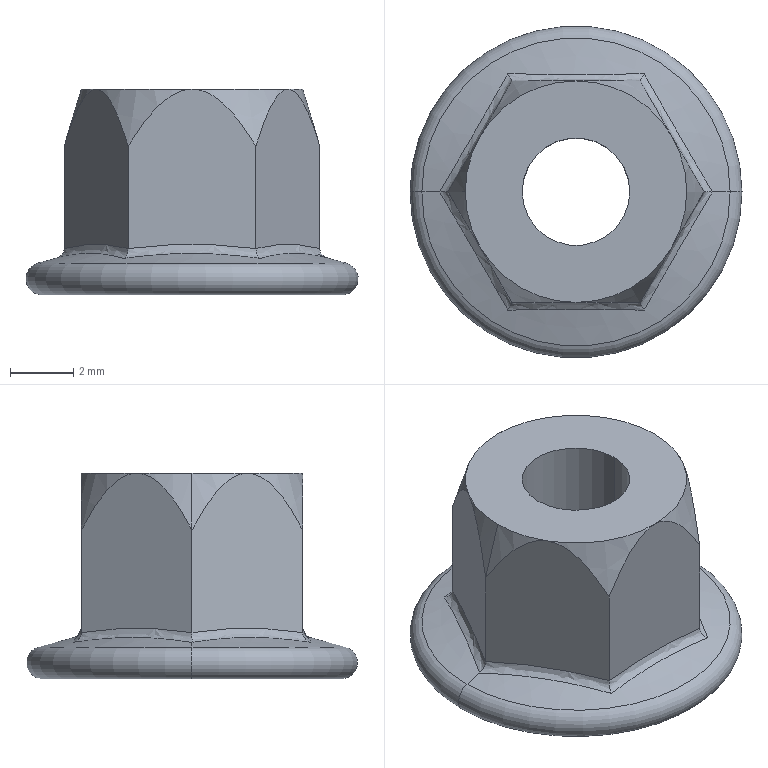Part | SolidWorks | features RevCut 2, Chamfer 1, Cut 1, Extrusion 1, Fillet 1, LPattern 1, Revolution 1 | 1 solid | 29 faces | box 10.5 x 10.5 x 6.5 mm | volume 259.355 mm3 | cone 11 | plane 8 | spline 6 | torus 2 | cylinder 2 | commonest cylinder face diameters 3.4 x2
STEP:
#1=CARTESIAN_POINT('',(2.155,3.733,-5.349));
#2=VERTEX_POINT('',#1);
#3=CARTESIAN_POINT('',(4.31,0.,-5.349));
#4=VERTEX_POINT('',#3);
#5=CARTESIAN_POINT('',(2.155,3.733,-5.349));
#6=CARTESIAN_POINT('',(2.508,3.111,-5.252));
#7=CARTESIAN_POINT('',(2.862,2.487,-5.192));
#8=CARTESIAN_POINT('',(3.584,1.237,-5.192));
#9=CARTESIAN_POINT('',(3.948,0.6165,-5.252));
#10=CARTESIAN_POINT('',(4.31,0.,-5.349));
#11=B_SPLINE_CURVE_WITH_KNOTS('',3,(#5,#6,#7,#8,#9,#10),.UNSPECIFIED.,.F.,.F.,(4,2,4),(0.,0.00216,0.004319),.UNSPECIFIED.);
#12=EDGE_CURVE('',#2,#4,#11,.T.);
#13=ORIENTED_EDGE('',*,*,#12,.T.);
#14=CARTESIAN_POINT('',(4.873,0.,-5.5));
#15=VERTEX_POINT('',#14);
#16=CARTESIAN_POINT('',(4.041,0.,-5.277));
#17=DIRECTION('',(0.9659,0.,-0.2588));
#18=VECTOR('',#17,1000.);
#19=LINE('',#16,#18);
#20=EDGE_CURVE('',#4,#15,#19,.T.);
#21=ORIENTED_EDGE('',*,*,#20,.T.);
#22=CARTESIAN_POINT('',(-4.873,0.,-5.5));
#23=VERTEX_POINT('',#22);
#24=CARTESIAN_POINT('',(0.,0.,-5.5));
#25=DIRECTION('',(0.,0.,-1.));
#26=DIRECTION('',(-1.,0.,0.));
#27=AXIS2_PLACEMENT_3D('',#24,#25,#26);
#28=CIRCLE('',#27,4.873);
#29=EDGE_CURVE('',#23,#15,#28,.T.);
#30=ORIENTED_EDGE('',*,*,#29,.F.);
#31=CARTESIAN_POINT('',(-4.31,0.,-5.349));
#32=VERTEX_POINT('',#31);
#33=CARTESIAN_POINT('',(-4.041,0.,-5.277));
#34=DIRECTION('',(-0.9659,0.,-0.2588));
#35=VECTOR('',#34,1000.);
#36=LINE('',#33,#35);
#37=EDGE_CURVE('',#32,#23,#36,.T.);
#38=ORIENTED_EDGE('',*,*,#37,.F.);
#39=CARTESIAN_POINT('',(-2.155,3.733,-5.349));
#40=VERTEX_POINT('',#39);
#41=CARTESIAN_POINT('',(-4.31,0.,-5.349));
#42=CARTESIAN_POINT('',(-3.948,0.6162,-5.252));
#43=CARTESIAN_POINT('',(-3.585,1.235,-5.192));
#44=CARTESIAN_POINT('',(-2.863,2.485,-5.192));
#45=CARTESIAN_POINT('',(-2.508,3.111,-5.252));
#46=CARTESIAN_POINT('',(-2.155,3.733,-5.349));
#47=B_SPLINE_CURVE_WITH_KNOTS('',3,(#41,#42,#43,#44,#45,#46),.UNSPECIFIED.,.F.,.F.,(4,2,4),(0.,0.00216,0.004319),.UNSPECIFIED.);
#48=EDGE_CURVE('',#32,#40,#47,.T.);
#49=ORIENTED_EDGE('',*,*,#48,.T.);
#50=CARTESIAN_POINT('',(-2.155,3.733,-5.349));
#51=CARTESIAN_POINT('',(-1.44,3.727,-5.252));
#52=CARTESIAN_POINT('',(-0.7231,3.722,-5.192));
#53=CARTESIAN_POINT('',(0.7205,3.722,-5.192));
#54=CARTESIAN_POINT('',(1.44,3.727,-5.252));
#55=CARTESIAN_POINT('',(2.155,3.733,-5.349));
#56=B_SPLINE_CURVE_WITH_KNOTS('',3,(#50,#51,#52,#53,#54,#55),.UNSPECIFIED.,.F.,.F.,(4,2,4),(0.,0.00216,0.004319),.UNSPECIFIED.);
#57=EDGE_CURVE('',#40,#2,#56,.T.);
#58=ORIENTED_EDGE('',*,*,#57,.T.);
#59=EDGE_LOOP('',(#13,#21,#30,#38,#49,#58));
#60=FACE_OUTER_BOUND('',#59,.T.);
#61=CARTESIAN_POINT('',(0.,0.,-5.277));
#62=DIRECTION('',(0.,0.,-1.));
#63=DIRECTION('',(-1.,0.,0.));
#64=AXIS2_PLACEMENT_3D('',#61,#62,#63);
#65=CONICAL_SURFACE('',#64,4.041,1.309);
#66=ADVANCED_FACE('',(#60),#65,.T.);
#67=ORIENTED_EDGE('',*,*,#29,.T.);
#68=CARTESIAN_POINT('',(4.741,0.,-6.5));
#69=VERTEX_POINT('',#68);
#70=CARTESIAN_POINT('',(4.741,0.,-5.991));
#71=DIRECTION('',(0.,1.,0.));
#72=DIRECTION('',(-1.,0.,0.));
#73=AXIS2_PLACEMENT_3D('',#70,#71,#72);
#74=CIRCLE('',#73,0.5087);
#75=EDGE_CURVE('',#15,#69,#74,.T.);
#76=ORIENTED_EDGE('',*,*,#75,.T.);
#77=CARTESIAN_POINT('',(-4.741,0.,-6.5));
#78=VERTEX_POINT('',#77);
#79=CARTESIAN_POINT('',(0.,0.,-6.5));
#80=DIRECTION('',(0.,0.,-1.));
#81=DIRECTION('',(-1.,0.,0.));
#82=AXIS2_PLACEMENT_3D('',#79,#80,#81);
#83=CIRCLE('',#82,4.741);
#84=EDGE_CURVE('',#78,#69,#83,.T.);
#85=ORIENTED_EDGE('',*,*,#84,.F.);
#86=CARTESIAN_POINT('',(-4.741,0.,-5.991));
#87=DIRECTION('',(0.,-1.,0.));
#88=DIRECTION('',(0.,0.,-1.));
#89=AXIS2_PLACEMENT_3D('',#86,#87,#88);
#90=CIRCLE('',#89,0.5087);
#91=EDGE_CURVE('',#23,#78,#90,.T.);
#92=ORIENTED_EDGE('',*,*,#91,.F.);
#93=EDGE_LOOP('',(#67,#76,#85,#92));
#94=FACE_OUTER_BOUND('',#93,.T.);
#95=CARTESIAN_POINT('',(0.,0.,-5.991));
#96=DIRECTION('',(0.,0.,-1.));
#97=DIRECTION('',(-1.,0.,0.));
#98=AXIS2_PLACEMENT_3D('',#95,#96,#97);
#99=TOROIDAL_SURFACE('',#98,4.741,0.5087);
#100=ADVANCED_FACE('',(#94),#99,.T.);
#101=CARTESIAN_POINT('',(1.7,0.,-6.014));
#102=VERTEX_POINT('',#101);
#103=CARTESIAN_POINT('',(-1.7,0.,-6.014));
#104=VERTEX_POINT('',#103);
#105=CARTESIAN_POINT('',(0.,0.,-6.014));
#106=DIRECTION('',(0.,0.,-1.));
#107=DIRECTION('',(1.,0.,0.));
#108=AXIS2_PLACEMENT_3D('',#105,#106,#107);
#109=CIRCLE('',#108,1.7);
#110=EDGE_CURVE('',#102,#104,#109,.T.);
#111=ORIENTED_EDGE('',*,*,#110,.F.);
#112=CARTESIAN_POINT('',(2.186,0.,-6.5));
#113=VERTEX_POINT('',#112);
#114=CARTESIAN_POINT('',(2.186,0.,-6.5));
#115=DIRECTION('',(0.7071,0.,-0.7071));
#116=VECTOR('',#115,1000.);
#117=LINE('',#114,#116);
#118=EDGE_CURVE('',#102,#113,#117,.T.);
#119=ORIENTED_EDGE('',*,*,#118,.T.);
#120=CARTESIAN_POINT('',(-2.186,0.,-6.5));
#121=VERTEX_POINT('',#120);
#122=CARTESIAN_POINT('',(0.,0.,-6.5));
#123=DIRECTION('',(0.,0.,1.));
#124=DIRECTION('',(1.,0.,0.));
#125=AXIS2_PLACEMENT_3D('',#122,#123,#124);
#126=CIRCLE('',#125,2.186);
#127=EDGE_CURVE('',#121,#113,#126,.T.);
#128=ORIENTED_EDGE('',*,*,#127,.F.);
#129=CARTESIAN_POINT('',(-2.186,0.,-6.5));
#130=DIRECTION('',(-0.7071,0.,-0.7071));
#131=VECTOR('',#130,1000.);
#132=LINE('',#129,#131);
#133=EDGE_CURVE('',#104,#121,#132,.T.);
#134=ORIENTED_EDGE('',*,*,#133,.F.);
#135=EDGE_LOOP('',(#111,#119,#128,#134));
#136=FACE_OUTER_BOUND('',#135,.T.);
#137=CARTESIAN_POINT('',(0.,0.,-6.5));
#138=DIRECTION('',(0.,0.,-1.));
#139=DIRECTION('',(-1.,0.,0.));
#140=AXIS2_PLACEMENT_3D('',#137,#138,#139);
#141=CONICAL_SURFACE('',#140,2.186,0.7854);
#142=ADVANCED_FACE('',(#136),#141,.F.);
#143=ORIENTED_EDGE('',*,*,#110,.T.);
#144=CARTESIAN_POINT('',(-1.7,0.,0.));
#145=VERTEX_POINT('',#144);
#146=CARTESIAN_POINT('',(-1.7,0.,-6.5));
#147=DIRECTION('',(0.,0.,1.));
#148=VECTOR('',#147,1000.);
#149=LINE('',#146,#148);
#150=EDGE_CURVE('',#104,#145,#149,.T.);
#151=ORIENTED_EDGE('',*,*,#150,.T.);
#152=CARTESIAN_POINT('',(1.7,0.,0.));
#153=VERTEX_POINT('',#152);
#154=CARTESIAN_POINT('',(0.,0.,0.));
#155=DIRECTION('',(0.,0.,1.));
#156=DIRECTION('',(1.,0.,0.));
#157=AXIS2_PLACEMENT_3D('',#154,#155,#156);
#158=CIRCLE('',#157,1.7);
#159=EDGE_CURVE('',#145,#153,#158,.T.);
#160=ORIENTED_EDGE('',*,*,#159,.T.);
#161=CARTESIAN_POINT('',(1.7,0.,-6.5));
#162=DIRECTION('',(0.,0.,1.));
#163=VECTOR('',#162,1000.);
#164=LINE('',#161,#163);
#165=EDGE_CURVE('',#102,#153,#164,.T.);
#166=ORIENTED_EDGE('',*,*,#165,.F.);
#167=EDGE_LOOP('',(#143,#151,#160,#166));
#168=FACE_OUTER_BOUND('',#167,.T.);
#169=CARTESIAN_POINT('',(0.,0.,-6.5));
#170=DIRECTION('',(0.,0.,1.));
#171=DIRECTION('',(1.,0.,0.));
#172=AXIS2_PLACEMENT_3D('',#169,#170,#171);
#173=CYLINDRICAL_SURFACE('',#172,1.7);
#174=ADVANCED_FACE('',(#168),#173,.F.);
#175=CARTESIAN_POINT('',(-3.031,-1.75,0.));
#176=VERTEX_POINT('',#175);
#177=CARTESIAN_POINT('',(-3.5,0.,0.));
#178=VERTEX_POINT('',#177);
#179=CARTESIAN_POINT('',(0.,0.,0.));
#180=DIRECTION('',(0.,0.,-1.));
#181=DIRECTION('',(1.,0.,0.));
#182=AXIS2_PLACEMENT_3D('',#179,#180,#181);
#183=CIRCLE('',#182,3.5);
#184=EDGE_CURVE('',#176,#178,#183,.T.);
#185=ORIENTED_EDGE('',*,*,#184,.T.);
#186=CARTESIAN_POINT('',(-4.041,0.,-1.8));
#187=VERTEX_POINT('',#186);
#188=CARTESIAN_POINT('',(-3.5,0.,0.));
#189=DIRECTION('',(-0.2881,0.,-0.9576));
#190=VECTOR('',#189,1000.);
#191=LINE('',#188,#190);
#192=EDGE_CURVE('',#178,#187,#191,.T.);
#193=ORIENTED_EDGE('',*,*,#192,.T.);
#194=CARTESIAN_POINT('',(-4.041,0.,-1.8));
#195=CARTESIAN_POINT('',(-3.981,-0.1048,-1.599));
#196=CARTESIAN_POINT('',(-3.918,-0.2143,-1.402));
#197=CARTESIAN_POINT('',(-3.783,-0.4485,-1.021));
#198=CARTESIAN_POINT('',(-3.711,-0.5729,-0.8364));
#199=CARTESIAN_POINT('',(-3.551,-0.8499,-0.4918));
#200=CARTESIAN_POINT('',(-3.463,-1.002,-0.3309));
#201=CARTESIAN_POINT('',(-3.313,-1.262,-0.1453));
#202=CARTESIAN_POINT('',(-3.26,-1.353,-0.09372));
#203=CARTESIAN_POINT('',(-3.149,-1.546,-0.02051));
#204=CARTESIAN_POINT('',(-3.09,-1.648,0.));
#205=CARTESIAN_POINT('',(-3.031,-1.75,0.));
#206=B_SPLINE_CURVE_WITH_KNOTS('',3,(#194,#195,#196,#197,#198,#199,#200,#201,#202,#203,#204,#205),.UNSPECIFIED.,.F.,.F.,(4,2,2,2,2,4),(0.000000232,0.0007011,0.001402,0.002103,0.002453,0.002804),.UNSPECIFIED.);
#207=EDGE_CURVE('',#187,#176,#206,.T.);
#208=ORIENTED_EDGE('',*,*,#207,.T.);
#209=EDGE_LOOP('',(#185,#193,#208));
#210=FACE_OUTER_BOUND('',#209,.T.);
#211=CARTESIAN_POINT('',(0.,0.,0.));
#212=DIRECTION('',(0.,0.,-1.));
#213=DIRECTION('',(-1.,0.,0.));
#214=AXIS2_PLACEMENT_3D('',#211,#212,#213);
#215=CONICAL_SURFACE('',#214,3.5,0.2922);
#216=ADVANCED_FACE('',(#210),#215,.T.);
#217=CARTESIAN_POINT('',(2.021,-3.5,-5.037));
#218=VERTEX_POINT('',#217);
#219=CARTESIAN_POINT('',(2.021,-3.5,-1.8));
#220=VERTEX_POINT('',#219);
#221=CARTESIAN_POINT('',(2.021,-3.5,-6.5));
#222=DIRECTION('',(0.,0.,1.));
#223=VECTOR('',#222,1000.);
#224=LINE('',#221,#223);
#225=EDGE_CURVE('',#218,#220,#224,.T.);
#226=ORIENTED_EDGE('',*,*,#225,.F.);
#227=CARTESIAN_POINT('',(4.041,0.,-5.037));
#228=VERTEX_POINT('',#227);
#229=CARTESIAN_POINT('',(2.021,-3.5,-5.037));
#230=CARTESIAN_POINT('',(2.356,-2.919,-4.953));
#231=CARTESIAN_POINT('',(2.693,-2.336,-4.902));
#232=CARTESIAN_POINT('',(3.369,-1.164,-4.902));
#233=CARTESIAN_POINT('',(3.706,-0.5811,-4.953));
#234=CARTESIAN_POINT('',(4.041,0.,-5.037));
#235=B_SPLINE_CURVE_WITH_KNOTS('',3,(#229,#230,#231,#232,#233,#234),.UNSPECIFIED.,.F.,.F.,(4,2,4),(0.,0.002025,0.00405),.UNSPECIFIED.);
#236=EDGE_CURVE('',#218,#228,#235,.T.);
#237=ORIENTED_EDGE('',*,*,#236,.T.);
#238=CARTESIAN_POINT('',(4.041,0.,-1.8));
#239=VERTEX_POINT('',#238);
#240=CARTESIAN_POINT('',(4.041,0.,-6.5));
#241=DIRECTION('',(0.,0.,1.));
#242=VECTOR('',#241,1000.);
#243=LINE('',#240,#242);
#244=EDGE_CURVE('',#228,#239,#243,.T.);
#245=ORIENTED_EDGE('',*,*,#244,.T.);
#246=CARTESIAN_POINT('',(3.031,-1.75,0.));
#247=VERTEX_POINT('',#246);
#248=CARTESIAN_POINT('',(3.031,-1.75,0.));
#249=CARTESIAN_POINT('',(3.09,-1.648,0.));
#250=CARTESIAN_POINT('',(3.149,-1.545,-0.02068));
#251=CARTESIAN_POINT('',(3.262,-1.351,-0.09464));
#252=CARTESIAN_POINT('',(3.315,-1.258,-0.148));
#253=CARTESIAN_POINT('',(3.465,-0.9986,-0.3345));
#254=CARTESIAN_POINT('',(3.553,-0.8457,-0.4965));
#255=CARTESIAN_POINT('',(3.712,-0.571,-0.8393));
#256=CARTESIAN_POINT('',(3.783,-0.4472,-1.023));
#257=CARTESIAN_POINT('',(3.918,-0.2138,-1.403));
#258=CARTESIAN_POINT('',(3.981,-0.1046,-1.599));
#259=CARTESIAN_POINT('',(4.041,0.,-1.8));
#260=B_SPLINE_CURVE_WITH_KNOTS('',3,(#248,#249,#250,#251,#252,#253,#254,#255,#256,#257,#258,#259),.UNSPECIFIED.,.F.,.F.,(4,2,2,2,2,4),(0.002804,0.003155,0.003507,0.00421,0.004914,0.005617),.UNSPECIFIED.);
#261=EDGE_CURVE('',#247,#239,#260,.T.);
#262=ORIENTED_EDGE('',*,*,#261,.F.);
#263=CARTESIAN_POINT('',(2.021,-3.5,-1.8));
#264=CARTESIAN_POINT('',(2.081,-3.395,-1.599));
#265=CARTESIAN_POINT('',(2.144,-3.286,-1.402));
#266=CARTESIAN_POINT('',(2.28,-3.052,-1.021));
#267=CARTESIAN_POINT('',(2.351,-2.927,-0.8364));
#268=CARTESIAN_POINT('',(2.511,-2.65,-0.4918));
#269=CARTESIAN_POINT('',(2.599,-2.498,-0.3309));
#270=CARTESIAN_POINT('',(2.749,-2.238,-0.1453));
#271=CARTESIAN_POINT('',(2.802,-2.147,-0.09372));
#272=CARTESIAN_POINT('',(2.913,-1.954,-0.02051));
#273=CARTESIAN_POINT('',(2.972,-1.852,0.));
#274=CARTESIAN_POINT('',(3.031,-1.75,0.));
#275=B_SPLINE_CURVE_WITH_KNOTS('',3,(#263,#264,#265,#266,#267,#268,#269,#270,#271,#272,#273,#274),.UNSPECIFIED.,.F.,.F.,(4,2,2,2,2,4),(0.000000232,0.0007011,0.001402,0.002103,0.002453,0.002804),.UNSPECIFIED.);
#276=EDGE_CURVE('',#220,#247,#275,.T.);
#277=ORIENTED_EDGE('',*,*,#276,.F.);
#278=EDGE_LOOP('',(#226,#237,#245,#262,#277));
#279=FACE_OUTER_BOUND('',#278,.T.);
#280=CARTESIAN_POINT('',(2.021,-3.5,-6.5));
#281=DIRECTION('',(0.866,-0.5,0.));
#282=DIRECTION('',(0.5,0.866,0.));
#283=AXIS2_PLACEMENT_3D('',#280,#281,#282);
#284=PLANE('',#283);
#285=ADVANCED_FACE('',(#279),#284,.T.);
#286=CARTESIAN_POINT('',(-2.021,-3.5,-5.037));
#287=VERTEX_POINT('',#286);
#288=CARTESIAN_POINT('',(-2.021,-3.5,-1.8));
#289=VERTEX_POINT('',#288);
#290=CARTESIAN_POINT('',(-2.021,-3.5,-6.5));
#291=DIRECTION('',(0.,0.,1.));
#292=VECTOR('',#291,1000.);
#293=LINE('',#290,#292);
#294=EDGE_CURVE('',#287,#289,#293,.T.);
#295=ORIENTED_EDGE('',*,*,#294,.F.);
#296=CARTESIAN_POINT('',(-2.021,-3.5,-5.037));
#297=CARTESIAN_POINT('',(-1.35,-3.5,-4.953));
#298=CARTESIAN_POINT('',(-0.6766,-3.5,-4.902));
#299=CARTESIAN_POINT('',(0.6766,-3.5,-4.902));
#300=CARTESIAN_POINT('',(1.35,-3.5,-4.953));
#301=CARTESIAN_POINT('',(2.021,-3.5,-5.037));
#302=B_SPLINE_CURVE_WITH_KNOTS('',3,(#296,#297,#298,#299,#300,#301),.UNSPECIFIED.,.F.,.F.,(4,2,4),(0.,0.002025,0.00405),.UNSPECIFIED.);
#303=EDGE_CURVE('',#287,#218,#302,.T.);
#304=ORIENTED_EDGE('',*,*,#303,.T.);
#305=ORIENTED_EDGE('',*,*,#225,.T.);
#306=CARTESIAN_POINT('',(0.,-3.5,0.));
#307=VERTEX_POINT('',#306);
#308=CARTESIAN_POINT('',(0.,-3.5,0.));
#309=CARTESIAN_POINT('',(0.118,-3.5,0.));
#310=CARTESIAN_POINT('',(0.234,-3.5,-0.01997));
#311=CARTESIAN_POINT('',(0.4599,-3.5,-0.09407));
#312=CARTESIAN_POINT('',(0.5651,-3.5,-0.1462));
#313=CARTESIAN_POINT('',(0.7651,-3.5,-0.2703));
#314=CARTESIAN_POINT('',(0.8598,-3.5,-0.3426));
#315=CARTESIAN_POINT('',(1.037,-3.5,-0.4965));
#316=CARTESIAN_POINT('',(1.12,-3.5,-0.5787));
#317=CARTESIAN_POINT('',(1.359,-3.5,-0.8363));
#318=CARTESIAN_POINT('',(1.505,-3.5,-1.023));
#319=CARTESIAN_POINT('',(1.775,-3.5,-1.405));
#320=CARTESIAN_POINT('',(1.901,-3.5,-1.601));
#321=CARTESIAN_POINT('',(2.021,-3.5,-1.8));
#322=B_SPLINE_CURVE_WITH_KNOTS('',3,(#308,#309,#310,#311,#312,#313,#314,#315,#316,#317,#318,#319,#320,#321),.UNSPECIFIED.,.F.,.F.,(4,2,2,2,2,2,4),(0.00757,0.007919,0.008268,0.008616,0.008965,0.009663,0.01036),.UNSPECIFIED.);
#323=EDGE_CURVE('',#307,#220,#322,.T.);
#324=ORIENTED_EDGE('',*,*,#323,.F.);
#325=CARTESIAN_POINT('',(-2.021,-3.5,-1.8));
#326=CARTESIAN_POINT('',(-1.901,-3.5,-1.6));
#327=CARTESIAN_POINT('',(-1.774,-3.5,-1.403));
#328=CARTESIAN_POINT('',(-1.502,-3.5,-1.02));
#329=CARTESIAN_POINT('',(-1.358,-3.5,-0.8356));
#330=CARTESIAN_POINT('',(-1.04,-3.5,-0.4928));
#331=CARTESIAN_POINT('',(-0.8644,-3.5,-0.3318));
#332=CARTESIAN_POINT('',(-0.5645,-3.5,-0.1458));
#333=CARTESIAN_POINT('',(-0.4572,-3.5,-0.0931));
#334=CARTESIAN_POINT('',(-0.2354,-3.5,-0.02053));
#335=CARTESIAN_POINT('',(-0.1178,-3.5,0.));
#336=CARTESIAN_POINT('',(0.,-3.5,0.));
#337=B_SPLINE_CURVE_WITH_KNOTS('',3,(#325,#326,#327,#328,#329,#330,#331,#332,#333,#334,#335,#336),.UNSPECIFIED.,.F.,.F.,(4,2,2,2,2,4),(0.004785,0.005481,0.006177,0.006874,0.007222,0.00757),.UNSPECIFIED.);
#338=EDGE_CURVE('',#289,#307,#337,.T.);
#339=ORIENTED_EDGE('',*,*,#338,.F.);
#340=EDGE_LOOP('',(#295,#304,#305,#324,#339));
#341=FACE_OUTER_BOUND('',#340,.T.);
#342=CARTESIAN_POINT('',(-2.021,-3.5,-6.5));
#343=DIRECTION('',(0.,-1.,0.));
#344=DIRECTION('',(1.,0.,0.));
#345=AXIS2_PLACEMENT_3D('',#342,#343,#344);
#346=PLANE('',#345);
#347=ADVANCED_FACE('',(#341),#346,.T.);
#348=CARTESIAN_POINT('',(-4.041,0.,-5.037));
#349=VERTEX_POINT('',#348);
#350=CARTESIAN_POINT('',(-4.041,0.,-6.5));
#351=DIRECTION('',(0.,0.,1.));
#352=VECTOR('',#351,1000.);
#353=LINE('',#350,#352);
#354=EDGE_CURVE('',#349,#187,#353,.T.);
#355=ORIENTED_EDGE('',*,*,#354,.F.);
#356=CARTESIAN_POINT('',(-4.041,0.,-5.037));
#357=CARTESIAN_POINT('',(-3.706,-0.5811,-4.953));
#358=CARTESIAN_POINT('',(-3.369,-1.164,-4.902));
#359=CARTESIAN_POINT('',(-2.693,-2.336,-4.902));
#360=CARTESIAN_POINT('',(-2.356,-2.919,-4.953));
#361=CARTESIAN_POINT('',(-2.021,-3.5,-5.037));
#362=B_SPLINE_CURVE_WITH_KNOTS('',3,(#356,#357,#358,#359,#360,#361),.UNSPECIFIED.,.F.,.F.,(4,2,4),(0.,0.002025,0.00405),.UNSPECIFIED.);
#363=EDGE_CURVE('',#349,#287,#362,.T.);
#364=ORIENTED_EDGE('',*,*,#363,.T.);
#365=ORIENTED_EDGE('',*,*,#294,.T.);
#366=CARTESIAN_POINT('',(-3.031,-1.75,0.));
#367=CARTESIAN_POINT('',(-2.972,-1.852,0.));
#368=CARTESIAN_POINT('',(-2.913,-1.955,-0.02068));
#369=CARTESIAN_POINT('',(-2.801,-2.149,-0.09464));
#370=CARTESIAN_POINT('',(-2.747,-2.242,-0.148));
#371=CARTESIAN_POINT('',(-2.597,-2.501,-0.3345));
#372=CARTESIAN_POINT('',(-2.509,-2.654,-0.4965));
#373=CARTESIAN_POINT('',(-2.35,-2.929,-0.8393));
#374=CARTESIAN_POINT('',(-2.279,-3.053,-1.023));
#375=CARTESIAN_POINT('',(-2.144,-3.286,-1.403));
#376=CARTESIAN_POINT('',(-2.081,-3.395,-1.599));
#377=CARTESIAN_POINT('',(-2.021,-3.5,-1.8));
#378=B_SPLINE_CURVE_WITH_KNOTS('',3,(#366,#367,#368,#369,#370,#371,#372,#373,#374,#375,#376,#377),.UNSPECIFIED.,.F.,.F.,(4,2,2,2,2,4),(0.002804,0.003155,0.003507,0.00421,0.004914,0.005617),.UNSPECIFIED.);
#379=EDGE_CURVE('',#176,#289,#378,.T.);
#380=ORIENTED_EDGE('',*,*,#379,.F.);
#381=ORIENTED_EDGE('',*,*,#207,.F.);
#382=EDGE_LOOP('',(#355,#364,#365,#380,#381));
#383=FACE_OUTER_BOUND('',#382,.T.);
#384=CARTESIAN_POINT('',(-4.041,0.,-6.5));
#385=DIRECTION('',(-0.866,-0.5,0.));
#386=DIRECTION('',(0.5,-0.866,0.));
#387=AXIS2_PLACEMENT_3D('',#384,#385,#386);
#388=PLANE('',#387);
#389=ADVANCED_FACE('',(#383),#388,.T.);
#390=CARTESIAN_POINT('',(-2.021,3.5,-5.037));
#391=VERTEX_POINT('',#390);
#392=CARTESIAN_POINT('',(-2.021,3.5,-1.8));
#393=VERTEX_POINT('',#392);
#394=CARTESIAN_POINT('',(-2.021,3.5,-6.5));
#395=DIRECTION('',(0.,0.,1.));
#396=VECTOR('',#395,1000.);
#397=LINE('',#394,#396);
#398=EDGE_CURVE('',#391,#393,#397,.T.);
#399=ORIENTED_EDGE('',*,*,#398,.F.);
#400=CARTESIAN_POINT('',(-2.021,3.5,-5.037));
#401=CARTESIAN_POINT('',(-2.356,2.919,-4.953));
#402=CARTESIAN_POINT('',(-2.693,2.336,-4.902));
#403=CARTESIAN_POINT('',(-3.369,1.164,-4.902));
#404=CARTESIAN_POINT('',(-3.706,0.5811,-4.953));
#405=CARTESIAN_POINT('',(-4.041,0.,-5.037));
#406=B_SPLINE_CURVE_WITH_KNOTS('',3,(#400,#401,#402,#403,#404,#405),.UNSPECIFIED.,.F.,.F.,(4,2,4),(0.,0.002025,0.00405),.UNSPECIFIED.);
#407=EDGE_CURVE('',#391,#349,#406,.T.);
#408=ORIENTED_EDGE('',*,*,#407,.T.);
#409=ORIENTED_EDGE('',*,*,#354,.T.);
#410=CARTESIAN_POINT('',(-3.031,1.75,0.));
#411=VERTEX_POINT('',#410);
#412=CARTESIAN_POINT('',(-3.031,1.75,0.));
#413=CARTESIAN_POINT('',(-3.09,1.648,0.));
#414=CARTESIAN_POINT('',(-3.149,1.545,-0.02068));
#415=CARTESIAN_POINT('',(-3.262,1.351,-0.09464));
#416=CARTESIAN_POINT('',(-3.315,1.258,-0.148));
#417=CARTESIAN_POINT('',(-3.465,0.9986,-0.3345));
#418=CARTESIAN_POINT('',(-3.553,0.8457,-0.4965));
#419=CARTESIAN_POINT('',(-3.712,0.571,-0.8393));
#420=CARTESIAN_POINT('',(-3.783,0.4472,-1.023));
#421=CARTESIAN_POINT('',(-3.918,0.2138,-1.403));
#422=CARTESIAN_POINT('',(-3.981,0.1046,-1.599));
#423=CARTESIAN_POINT('',(-4.041,0.,-1.8));
#424=B_SPLINE_CURVE_WITH_KNOTS('',3,(#412,#413,#414,#415,#416,#417,#418,#419,#420,#421,#422,#423),.UNSPECIFIED.,.F.,.F.,(4,2,2,2,2,4),(0.002804,0.003155,0.003507,0.00421,0.004914,0.005617),.UNSPECIFIED.);
#425=EDGE_CURVE('',#411,#187,#424,.T.);
#426=ORIENTED_EDGE('',*,*,#425,.F.);
#427=CARTESIAN_POINT('',(-2.021,3.5,-1.8));
#428=CARTESIAN_POINT('',(-2.081,3.395,-1.599));
#429=CARTESIAN_POINT('',(-2.144,3.286,-1.402));
#430=CARTESIAN_POINT('',(-2.28,3.052,-1.021));
#431=CARTESIAN_POINT('',(-2.351,2.927,-0.8364));
#432=CARTESIAN_POINT('',(-2.511,2.65,-0.4918));
#433=CARTESIAN_POINT('',(-2.599,2.498,-0.3309));
#434=CARTESIAN_POINT('',(-2.749,2.238,-0.1453));
#435=CARTESIAN_POINT('',(-2.802,2.147,-0.09372));
#436=CARTESIAN_POINT('',(-2.913,1.954,-0.02051));
#437=CARTESIAN_POINT('',(-2.972,1.852,0.));
#438=CARTESIAN_POINT('',(-3.031,1.75,0.));
#439=B_SPLINE_CURVE_WITH_KNOTS('',3,(#427,#428,#429,#430,#431,#432,#433,#434,#435,#436,#437,#438),.UNSPECIFIED.,.F.,.F.,(4,2,2,2,2,4),(0.000000232,0.0007011,0.001402,0.002103,0.002453,0.002804),.UNSPECIFIED.);
#440=EDGE_CURVE('',#393,#411,#439,.T.);
#441=ORIENTED_EDGE('',*,*,#440,.F.);
#442=EDGE_LOOP('',(#399,#408,#409,#426,#441));
#443=FACE_OUTER_BOUND('',#442,.T.);
#444=CARTESIAN_POINT('',(-2.021,3.5,-6.5));
#445=DIRECTION('',(-0.866,0.5,0.));
#446=DIRECTION('',(-0.5,-0.866,0.));
#447=AXIS2_PLACEMENT_3D('',#444,#445,#446);
#448=PLANE('',#447);
#449=ADVANCED_FACE('',(#443),#448,.T.);
#450=CARTESIAN_POINT('',(2.021,3.5,-5.037));
#451=VERTEX_POINT('',#450);
#452=CARTESIAN_POINT('',(2.021,3.5,-1.8));
#453=VERTEX_POINT('',#452);
#454=CARTESIAN_POINT('',(2.021,3.5,-6.5));
#455=DIRECTION('',(0.,0.,1.));
#456=VECTOR('',#455,1000.);
#457=LINE('',#454,#456);
#458=EDGE_CURVE('',#451,#453,#457,.T.);
#459=ORIENTED_EDGE('',*,*,#458,.F.);
#460=CARTESIAN_POINT('',(2.021,3.5,-5.037));
#461=CARTESIAN_POINT('',(1.35,3.5,-4.953));
#462=CARTESIAN_POINT('',(0.6766,3.5,-4.902));
#463=CARTESIAN_POINT('',(-0.6766,3.5,-4.902));
#464=CARTESIAN_POINT('',(-1.35,3.5,-4.953));
#465=CARTESIAN_POINT('',(-2.021,3.5,-5.037));
#466=B_SPLINE_CURVE_WITH_KNOTS('',3,(#460,#461,#462,#463,#464,#465),.UNSPECIFIED.,.F.,.F.,(4,2,4),(0.,0.002025,0.00405),.UNSPECIFIED.);
#467=EDGE_CURVE('',#451,#391,#466,.T.);
#468=ORIENTED_EDGE('',*,*,#467,.T.);
#469=ORIENTED_EDGE('',*,*,#398,.T.);
#470=CARTESIAN_POINT('',(0.,3.5,0.));
#471=VERTEX_POINT('',#470);
#472=CARTESIAN_POINT('',(0.,3.5,0.));
#473=CARTESIAN_POINT('',(-0.1178,3.5,0.));
#474=CARTESIAN_POINT('',(-0.2354,3.5,-0.02053));
#475=CARTESIAN_POINT('',(-0.4572,3.5,-0.0931));
#476=CARTESIAN_POINT('',(-0.5645,3.5,-0.1458));
#477=CARTESIAN_POINT('',(-0.8644,3.5,-0.3318));
#478=CARTESIAN_POINT('',(-1.04,3.5,-0.4928));
#479=CARTESIAN_POINT('',(-1.358,3.5,-0.8356));
#480=CARTESIAN_POINT('',(-1.502,3.5,-1.02));
#481=CARTESIAN_POINT('',(-1.774,3.5,-1.403));
#482=CARTESIAN_POINT('',(-1.901,3.5,-1.6));
#483=CARTESIAN_POINT('',(-2.021,3.5,-1.8));
#484=B_SPLINE_CURVE_WITH_KNOTS('',3,(#472,#473,#474,#475,#476,#477,#478,#479,#480,#481,#482,#483),.UNSPECIFIED.,.F.,.F.,(4,2,2,2,2,4),(0.005451,0.005799,0.006147,0.006843,0.007539,0.008235),.UNSPECIFIED.);
#485=EDGE_CURVE('',#471,#393,#484,.T.);
#486=ORIENTED_EDGE('',*,*,#485,.F.);
#487=CARTESIAN_POINT('',(2.021,3.5,-1.8));
#488=CARTESIAN_POINT('',(1.901,3.5,-1.601));
#489=CARTESIAN_POINT('',(1.775,3.5,-1.405));
#490=CARTESIAN_POINT('',(1.505,3.5,-1.023));
#491=CARTESIAN_POINT('',(1.359,3.5,-0.8363));
#492=CARTESIAN_POINT('',(1.12,3.5,-0.5787));
#493=CARTESIAN_POINT('',(1.037,3.5,-0.4965));
#494=CARTESIAN_POINT('',(0.8598,3.5,-0.3426));
#495=CARTESIAN_POINT('',(0.7651,3.5,-0.2703));
#496=CARTESIAN_POINT('',(0.5651,3.5,-0.1462));
#497=CARTESIAN_POINT('',(0.4599,3.5,-0.09407));
#498=CARTESIAN_POINT('',(0.234,3.5,-0.01997));
#499=CARTESIAN_POINT('',(0.118,3.5,0.));
#500=CARTESIAN_POINT('',(0.,3.5,0.));
#501=B_SPLINE_CURVE_WITH_KNOTS('',3,(#487,#488,#489,#490,#491,#492,#493,#494,#495,#496,#497,#498,#499,#500),.UNSPECIFIED.,.F.,.F.,(4,2,2,2,2,2,4),(0.002663,0.00336,0.004057,0.004406,0.004754,0.005103,0.005451),.UNSPECIFIED.);
#502=EDGE_CURVE('',#453,#471,#501,.T.);
#503=ORIENTED_EDGE('',*,*,#502,.F.);
#504=EDGE_LOOP('',(#459,#468,#469,#486,#503));
#505=FACE_OUTER_BOUND('',#504,.T.);
#506=CARTESIAN_POINT('',(2.021,3.5,-6.5));
#507=DIRECTION('',(0.,1.,0.));
#508=DIRECTION('',(-1.,0.,0.));
#509=AXIS2_PLACEMENT_3D('',#506,#507,#508);
#510=PLANE('',#509);
#511=ADVANCED_FACE('',(#505),#510,.T.);
#512=ORIENTED_EDGE('',*,*,#244,.F.);
#513=CARTESIAN_POINT('',(4.041,0.,-5.037));
#514=CARTESIAN_POINT('',(3.706,0.5811,-4.953));
#515=CARTESIAN_POINT('',(3.369,1.164,-4.902));
#516=CARTESIAN_POINT('',(2.693,2.336,-4.902));
#517=CARTESIAN_POINT('',(2.356,2.919,-4.953));
#518=CARTESIAN_POINT('',(2.021,3.5,-5.037));
#519=B_SPLINE_CURVE_WITH_KNOTS('',3,(#513,#514,#515,#516,#517,#518),.UNSPECIFIED.,.F.,.F.,(4,2,4),(0.,0.002025,0.00405),.UNSPECIFIED.);
#520=EDGE_CURVE('',#228,#451,#519,.T.);
#521=ORIENTED_EDGE('',*,*,#520,.T.);
#522=ORIENTED_EDGE('',*,*,#458,.T.);
#523=CARTESIAN_POINT('',(3.031,1.75,0.));
#524=VERTEX_POINT('',#523);
#525=CARTESIAN_POINT('',(3.031,1.75,0.));
#526=CARTESIAN_POINT('',(2.972,1.852,0.));
#527=CARTESIAN_POINT('',(2.913,1.955,-0.02068));
#528=CARTESIAN_POINT('',(2.801,2.149,-0.09464));
#529=CARTESIAN_POINT('',(2.747,2.242,-0.148));
#530=CARTESIAN_POINT('',(2.597,2.501,-0.3345));
#531=CARTESIAN_POINT('',(2.509,2.654,-0.4965));
#532=CARTESIAN_POINT('',(2.35,2.929,-0.8393));
#533=CARTESIAN_POINT('',(2.279,3.053,-1.023));
#534=CARTESIAN_POINT('',(2.144,3.286,-1.403));
#535=CARTESIAN_POINT('',(2.081,3.395,-1.599));
#536=CARTESIAN_POINT('',(2.021,3.5,-1.8));
#537=B_SPLINE_CURVE_WITH_KNOTS('',3,(#525,#526,#527,#528,#529,#530,#531,#532,#533,#534,#535,#536),.UNSPECIFIED.,.F.,.F.,(4,2,2,2,2,4),(0.002804,0.003155,0.003507,0.00421,0.004914,0.005617),.UNSPECIFIED.);
#538=EDGE_CURVE('',#524,#453,#537,.T.);
#539=ORIENTED_EDGE('',*,*,#538,.F.);
#540=CARTESIAN_POINT('',(4.041,0.,-1.8));
#541=CARTESIAN_POINT('',(3.981,0.1048,-1.599));
#542=CARTESIAN_POINT('',(3.918,0.2143,-1.402));
#543=CARTESIAN_POINT('',(3.783,0.4485,-1.021));
#544=CARTESIAN_POINT('',(3.711,0.5729,-0.8364));
#545=CARTESIAN_POINT('',(3.551,0.8499,-0.4918));
#546=CARTESIAN_POINT('',(3.463,1.002,-0.3309));
#547=CARTESIAN_POINT('',(3.313,1.262,-0.1453));
#548=CARTESIAN_POINT('',(3.26,1.353,-0.09372));
#549=CARTESIAN_POINT('',(3.149,1.546,-0.02051));
#550=CARTESIAN_POINT('',(3.09,1.648,0.));
#551=CARTESIAN_POINT('',(3.031,1.75,0.));
#552=B_SPLINE_CURVE_WITH_KNOTS('',3,(#540,#541,#542,#543,#544,#545,#546,#547,#548,#549,#550,#551),.UNSPECIFIED.,.F.,.F.,(4,2,2,2,2,4),(0.000000232,0.0007011,0.001402,0.002103,0.002453,0.002804),.UNSPECIFIED.);
#553=EDGE_CURVE('',#239,#524,#552,.T.);
#554=ORIENTED_EDGE('',*,*,#553,.F.);
#555=EDGE_LOOP('',(#512,#521,#522,#539,#554));
#556=FACE_OUTER_BOUND('',#555,.T.);
#557=CARTESIAN_POINT('',(4.041,0.,-6.5));
#558=DIRECTION('',(0.866,0.5,0.));
#559=DIRECTION('',(-0.5,0.866,0.));
#560=AXIS2_PLACEMENT_3D('',#557,#558,#559);
#561=PLANE('',#560);
#562=ADVANCED_FACE('',(#556),#561,.T.);
#563=ORIENTED_EDGE('',*,*,#127,.T.);
#564=CARTESIAN_POINT('',(0.,0.,-6.5));
#565=DIRECTION('',(0.,0.,1.));
#566=DIRECTION('',(1.,0.,0.));
#567=AXIS2_PLACEMENT_3D('',#564,#565,#566);
#568=CIRCLE('',#567,2.186);
#569=EDGE_CURVE('',#113,#121,#568,.T.);
#570=ORIENTED_EDGE('',*,*,#569,.T.);
#571=EDGE_LOOP('',(#563,#570));
#572=FACE_BOUND('',#571,.T.);
#573=ORIENTED_EDGE('',*,*,#84,.T.);
#574=CARTESIAN_POINT('',(0.,0.,-6.5));
#575=DIRECTION('',(0.,0.,-1.));
#576=DIRECTION('',(-1.,0.,0.));
#577=AXIS2_PLACEMENT_3D('',#574,#575,#576);
#578=CIRCLE('',#577,4.741);
#579=EDGE_CURVE('',#69,#78,#578,.T.);
#580=ORIENTED_EDGE('',*,*,#579,.T.);
#581=EDGE_LOOP('',(#573,#580));
#582=FACE_OUTER_BOUND('',#581,.T.);
#583=CARTESIAN_POINT('',(4.041,0.,-6.5));
#584=DIRECTION('',(0.,0.,1.));
#585=DIRECTION('',(1.,0.,0.));
#586=AXIS2_PLACEMENT_3D('',#583,#584,#585);
#587=PLANE('',#586);
#588=ADVANCED_FACE('',(#572,#582),#587,.F.);
#589=ORIENTED_EDGE('',*,*,#261,.T.);
#590=ORIENTED_EDGE('',*,*,#553,.T.);
#591=CARTESIAN_POINT('',(0.,0.,0.));
#592=DIRECTION('',(0.,0.,-1.));
#593=DIRECTION('',(1.,0.,0.));
#594=AXIS2_PLACEMENT_3D('',#591,#592,#593);
#595=CIRCLE('',#594,3.5);
#596=EDGE_CURVE('',#524,#247,#595,.T.);
#597=ORIENTED_EDGE('',*,*,#596,.T.);
#598=EDGE_LOOP('',(#589,#590,#597));
#599=FACE_OUTER_BOUND('',#598,.T.);
#600=CARTESIAN_POINT('',(0.,0.,0.));
#601=DIRECTION('',(0.,0.,-1.));
#602=DIRECTION('',(-1.,0.,0.));
#603=AXIS2_PLACEMENT_3D('',#600,#601,#602);
#604=CONICAL_SURFACE('',#603,3.5,0.2922);
#605=ADVANCED_FACE('',(#599),#604,.T.);
#606=ORIENTED_EDGE('',*,*,#502,.T.);
#607=CARTESIAN_POINT('',(0.,0.,0.));
#608=DIRECTION('',(0.,0.,-1.));
#609=DIRECTION('',(1.,0.,0.));
#610=AXIS2_PLACEMENT_3D('',#607,#608,#609);
#611=CIRCLE('',#610,3.5);
#612=EDGE_CURVE('',#471,#524,#611,.T.);
#613=ORIENTED_EDGE('',*,*,#612,.T.);
#614=ORIENTED_EDGE('',*,*,#538,.T.);
#615=EDGE_LOOP('',(#606,#613,#614));
#616=FACE_OUTER_BOUND('',#615,.T.);
#617=CARTESIAN_POINT('',(0.,0.,0.));
#618=DIRECTION('',(0.,0.,-1.));
#619=DIRECTION('',(-1.,0.,0.));
#620=AXIS2_PLACEMENT_3D('',#617,#618,#619);
#621=CONICAL_SURFACE('',#620,3.5,0.2922);
#622=ADVANCED_FACE('',(#616),#621,.T.);
#623=ORIENTED_EDGE('',*,*,#440,.T.);
#624=CARTESIAN_POINT('',(0.,0.,0.));
#625=DIRECTION('',(0.,0.,-1.));
#626=DIRECTION('',(-1.,0.,0.));
#627=AXIS2_PLACEMENT_3D('',#624,#625,#626);
#628=CIRCLE('',#627,3.5);
#629=EDGE_CURVE('',#411,#471,#628,.T.);
#630=ORIENTED_EDGE('',*,*,#629,.T.);
#631=ORIENTED_EDGE('',*,*,#485,.T.);
#632=EDGE_LOOP('',(#623,#630,#631));
#633=FACE_OUTER_BOUND('',#632,.T.);
#634=CARTESIAN_POINT('',(0.,0.,0.));
#635=DIRECTION('',(0.,0.,-1.));
#636=DIRECTION('',(-1.,0.,0.));
#637=AXIS2_PLACEMENT_3D('',#634,#635,#636);
#638=CONICAL_SURFACE('',#637,3.5,0.2922);
#639=ADVANCED_FACE('',(#633),#638,.T.);
#640=ORIENTED_EDGE('',*,*,#192,.F.);
#641=CARTESIAN_POINT('',(0.,0.,0.));
#642=DIRECTION('',(0.,0.,-1.));
#643=DIRECTION('',(1.,0.,0.));
#644=AXIS2_PLACEMENT_3D('',#641,#642,#643);
#645=CIRCLE('',#644,3.5);
#646=EDGE_CURVE('',#178,#411,#645,.T.);
#647=ORIENTED_EDGE('',*,*,#646,.T.);
#648=ORIENTED_EDGE('',*,*,#425,.T.);
#649=EDGE_LOOP('',(#640,#647,#648));
#650=FACE_OUTER_BOUND('',#649,.T.);
#651=CARTESIAN_POINT('',(0.,0.,0.));
#652=DIRECTION('',(0.,0.,-1.));
#653=DIRECTION('',(-1.,0.,0.));
#654=AXIS2_PLACEMENT_3D('',#651,#652,#653);
#655=CONICAL_SURFACE('',#654,3.5,0.2922);
#656=ADVANCED_FACE('',(#650),#655,.T.);
#657=ORIENTED_EDGE('',*,*,#379,.T.);
#658=ORIENTED_EDGE('',*,*,#338,.T.);
#659=CARTESIAN_POINT('',(0.,0.,0.));
#660=DIRECTION('',(0.,0.,-1.));
#661=DIRECTION('',(1.,0.,0.));
#662=AXIS2_PLACEMENT_3D('',#659,#660,#661);
#663=CIRCLE('',#662,3.5);
#664=EDGE_CURVE('',#307,#176,#663,.T.);
#665=ORIENTED_EDGE('',*,*,#664,.T.);
#666=EDGE_LOOP('',(#657,#658,#665));
#667=FACE_OUTER_BOUND('',#666,.T.);
#668=CARTESIAN_POINT('',(0.,0.,0.));
#669=DIRECTION('',(0.,0.,-1.));
#670=DIRECTION('',(-1.,0.,0.));
#671=AXIS2_PLACEMENT_3D('',#668,#669,#670);
#672=CONICAL_SURFACE('',#671,3.5,0.2922);
#673=ADVANCED_FACE('',(#667),#672,.T.);
#674=ORIENTED_EDGE('',*,*,#323,.T.);
#675=ORIENTED_EDGE('',*,*,#276,.T.);
#676=CARTESIAN_POINT('',(0.,0.,0.));
#677=DIRECTION('',(0.,0.,-1.));
#678=DIRECTION('',(1.,0.,0.));
#679=AXIS2_PLACEMENT_3D('',#676,#677,#678);
#680=CIRCLE('',#679,3.5);
#681=EDGE_CURVE('',#247,#307,#680,.T.);
#682=ORIENTED_EDGE('',*,*,#681,.T.);
#683=EDGE_LOOP('',(#674,#675,#682));
#684=FACE_OUTER_BOUND('',#683,.T.);
#685=CARTESIAN_POINT('',(0.,0.,0.));
#686=DIRECTION('',(0.,0.,-1.));
#687=DIRECTION('',(-1.,0.,0.));
#688=AXIS2_PLACEMENT_3D('',#685,#686,#687);
#689=CONICAL_SURFACE('',#688,3.5,0.2922);
#690=ADVANCED_FACE('',(#684),#689,.T.);
#691=CARTESIAN_POINT('',(0.,0.,0.));
#692=DIRECTION('',(0.,0.,1.));
#693=DIRECTION('',(1.,0.,0.));
#694=AXIS2_PLACEMENT_3D('',#691,#692,#693);
#695=CIRCLE('',#694,1.7);
#696=EDGE_CURVE('',#153,#145,#695,.T.);
#697=ORIENTED_EDGE('',*,*,#696,.F.);
#698=ORIENTED_EDGE('',*,*,#159,.F.);
#699=EDGE_LOOP('',(#697,#698));
#700=FACE_BOUND('',#699,.T.);
#701=ORIENTED_EDGE('',*,*,#681,.F.);
#702=ORIENTED_EDGE('',*,*,#596,.F.);
#703=ORIENTED_EDGE('',*,*,#612,.F.);
#704=ORIENTED_EDGE('',*,*,#629,.F.);
#705=ORIENTED_EDGE('',*,*,#646,.F.);
#706=ORIENTED_EDGE('',*,*,#184,.F.);
#707=ORIENTED_EDGE('',*,*,#664,.F.);
#708=EDGE_LOOP('',(#701,#702,#703,#704,#705,#706,#707));
#709=FACE_OUTER_BOUND('',#708,.T.);
#710=CARTESIAN_POINT('',(4.041,0.,0.));
#711=DIRECTION('',(0.,0.,1.));
#712=DIRECTION('',(1.,0.,0.));
#713=AXIS2_PLACEMENT_3D('',#710,#711,#712);
#714=PLANE('',#713);
#715=ADVANCED_FACE('',(#700,#709),#714,.T.);
#716=ORIENTED_EDGE('',*,*,#150,.F.);
#717=CARTESIAN_POINT('',(0.,0.,-6.014));
#718=DIRECTION('',(0.,0.,-1.));
#719=DIRECTION('',(1.,0.,0.));
#720=AXIS2_PLACEMENT_3D('',#717,#718,#719);
#721=CIRCLE('',#720,1.7);
#722=EDGE_CURVE('',#104,#102,#721,.T.);
#723=ORIENTED_EDGE('',*,*,#722,.T.);
#724=ORIENTED_EDGE('',*,*,#165,.T.);
#725=ORIENTED_EDGE('',*,*,#696,.T.);
#726=EDGE_LOOP('',(#716,#723,#724,#725));
#727=FACE_OUTER_BOUND('',#726,.T.);
#728=CARTESIAN_POINT('',(0.,0.,-6.5));
#729=DIRECTION('',(0.,0.,1.));
#730=DIRECTION('',(1.,0.,0.));
#731=AXIS2_PLACEMENT_3D('',#728,#729,#730);
#732=CYLINDRICAL_SURFACE('',#731,1.7);
#733=ADVANCED_FACE('',(#727),#732,.F.);
#734=ORIENTED_EDGE('',*,*,#118,.F.);
#735=ORIENTED_EDGE('',*,*,#722,.F.);
#736=ORIENTED_EDGE('',*,*,#133,.T.);
#737=ORIENTED_EDGE('',*,*,#569,.F.);
#738=EDGE_LOOP('',(#734,#735,#736,#737));
#739=FACE_OUTER_BOUND('',#738,.T.);
#740=CARTESIAN_POINT('',(0.,0.,-6.5));
#741=DIRECTION('',(0.,0.,-1.));
#742=DIRECTION('',(-1.,0.,0.));
#743=AXIS2_PLACEMENT_3D('',#740,#741,#742);
#744=CONICAL_SURFACE('',#743,2.186,0.7854);
#745=ADVANCED_FACE('',(#739),#744,.F.);
#746=ORIENTED_EDGE('',*,*,#75,.F.);
#747=CARTESIAN_POINT('',(0.,0.,-5.5));
#748=DIRECTION('',(0.,0.,-1.));
#749=DIRECTION('',(-1.,0.,0.));
#750=AXIS2_PLACEMENT_3D('',#747,#748,#749);
#751=CIRCLE('',#750,4.873);
#752=EDGE_CURVE('',#15,#23,#751,.T.);
#753=ORIENTED_EDGE('',*,*,#752,.T.);
#754=ORIENTED_EDGE('',*,*,#91,.T.);
#755=ORIENTED_EDGE('',*,*,#579,.F.);
#756=EDGE_LOOP('',(#746,#753,#754,#755));
#757=FACE_OUTER_BOUND('',#756,.T.);
#758=CARTESIAN_POINT('',(0.,0.,-5.991));
#759=DIRECTION('',(0.,0.,-1.));
#760=DIRECTION('',(-1.,0.,0.));
#761=AXIS2_PLACEMENT_3D('',#758,#759,#760);
#762=TOROIDAL_SURFACE('',#761,4.741,0.5087);
#763=ADVANCED_FACE('',(#757),#762,.T.);
#764=ORIENTED_EDGE('',*,*,#20,.F.);
#765=CARTESIAN_POINT('',(2.155,-3.733,-5.349));
#766=VERTEX_POINT('',#765);
#767=CARTESIAN_POINT('',(4.31,0.,-5.349));
#768=CARTESIAN_POINT('',(3.948,-0.6162,-5.252));
#769=CARTESIAN_POINT('',(3.585,-1.235,-5.192));
#770=CARTESIAN_POINT('',(2.863,-2.485,-5.192));
#771=CARTESIAN_POINT('',(2.508,-3.111,-5.252));
#772=CARTESIAN_POINT('',(2.155,-3.733,-5.349));
#773=B_SPLINE_CURVE_WITH_KNOTS('',3,(#767,#768,#769,#770,#771,#772),.UNSPECIFIED.,.F.,.F.,(4,2,4),(0.,0.00216,0.004319),.UNSPECIFIED.);
#774=EDGE_CURVE('',#4,#766,#773,.T.);
#775=ORIENTED_EDGE('',*,*,#774,.T.);
#776=CARTESIAN_POINT('',(-2.155,-3.733,-5.349));
#777=VERTEX_POINT('',#776);
#778=CARTESIAN_POINT('',(2.155,-3.733,-5.349));
#779=CARTESIAN_POINT('',(1.44,-3.727,-5.252));
#780=CARTESIAN_POINT('',(0.723,-3.722,-5.192));
#781=CARTESIAN_POINT('',(-0.7206,-3.722,-5.192));
#782=CARTESIAN_POINT('',(-1.44,-3.727,-5.252));
#783=CARTESIAN_POINT('',(-2.155,-3.733,-5.349));
#784=B_SPLINE_CURVE_WITH_KNOTS('',3,(#778,#779,#780,#781,#782,#783),.UNSPECIFIED.,.F.,.F.,(4,2,4),(0.,0.00216,0.004319),.UNSPECIFIED.);
#785=EDGE_CURVE('',#766,#777,#784,.T.);
#786=ORIENTED_EDGE('',*,*,#785,.T.);
#787=CARTESIAN_POINT('',(-2.155,-3.733,-5.349));
#788=CARTESIAN_POINT('',(-2.508,-3.111,-5.252));
#789=CARTESIAN_POINT('',(-2.862,-2.487,-5.192));
#790=CARTESIAN_POINT('',(-3.584,-1.237,-5.192));
#791=CARTESIAN_POINT('',(-3.948,-0.6165,-5.252));
#792=CARTESIAN_POINT('',(-4.31,0.,-5.349));
#793=B_SPLINE_CURVE_WITH_KNOTS('',3,(#787,#788,#789,#790,#791,#792),.UNSPECIFIED.,.F.,.F.,(4,2,4),(0.,0.00216,0.004319),.UNSPECIFIED.);
#794=EDGE_CURVE('',#777,#32,#793,.T.);
#795=ORIENTED_EDGE('',*,*,#794,.T.);
#796=ORIENTED_EDGE('',*,*,#37,.T.);
#797=ORIENTED_EDGE('',*,*,#752,.F.);
#798=EDGE_LOOP('',(#764,#775,#786,#795,#796,#797));
#799=FACE_OUTER_BOUND('',#798,.T.);
#800=CARTESIAN_POINT('',(0.,0.,-5.277));
#801=DIRECTION('',(0.,0.,-1.));
#802=DIRECTION('',(-1.,0.,0.));
#803=AXIS2_PLACEMENT_3D('',#800,#801,#802);
#804=CONICAL_SURFACE('',#803,4.041,1.309);
#805=ADVANCED_FACE('',(#799),#804,.T.);
#806=CARTESIAN_POINT('',(4.041,0.,-5.037));
#807=CARTESIAN_POINT('',(4.041,0.,-5.111));
#808=CARTESIAN_POINT('',(4.074,0.,-5.183));
#809=CARTESIAN_POINT('',(4.173,0.,-5.292));
#810=CARTESIAN_POINT('',(4.239,0.,-5.33));
#811=CARTESIAN_POINT('',(4.31,0.,-5.349));
#812=B_SPLINE_CURVE_WITH_KNOTS('',3,(#806,#807,#808,#809,#810,#811),.UNSPECIFIED.,.F.,.F.,(4,2,4),(0.,0.0002199,0.0004397),.UNSPECIFIED.);
#813=EDGE_CURVE('',#228,#4,#812,.T.);
#814=ORIENTED_EDGE('',*,*,#813,.F.);
#815=ORIENTED_EDGE('',*,*,#236,.F.);
#816=CARTESIAN_POINT('',(2.155,-3.733,-5.349));
#817=CARTESIAN_POINT('',(2.119,-3.671,-5.33));
#818=CARTESIAN_POINT('',(2.086,-3.614,-5.292));
#819=CARTESIAN_POINT('',(2.037,-3.528,-5.183));
#820=CARTESIAN_POINT('',(2.021,-3.5,-5.111));
#821=CARTESIAN_POINT('',(2.021,-3.5,-5.037));
#822=B_SPLINE_CURVE_WITH_KNOTS('',3,(#816,#817,#818,#819,#820,#821),.UNSPECIFIED.,.F.,.F.,(4,2,4),(-0.000003667,0.0002188,0.0004414),.UNSPECIFIED.);
#823=EDGE_CURVE('',#766,#218,#822,.T.);
#824=ORIENTED_EDGE('',*,*,#823,.F.);
#825=ORIENTED_EDGE('',*,*,#774,.F.);
#826=EDGE_LOOP('',(#814,#815,#824,#825));
#827=FACE_OUTER_BOUND('',#826,.T.);
#828=CARTESIAN_POINT('',(1.921,-3.672,-5.063));
#829=CARTESIAN_POINT('',(1.937,-3.645,-5.3));
#830=CARTESIAN_POINT('',(2.143,-3.755,-5.353));
#831=CARTESIAN_POINT('',(2.285,-3.043,-4.965));
#832=CARTESIAN_POINT('',(2.294,-3.027,-5.199));
#833=CARTESIAN_POINT('',(2.497,-3.131,-5.254));
#834=CARTESIAN_POINT('',(2.652,-2.406,-4.902));
#835=CARTESIAN_POINT('',(2.658,-2.395,-5.133));
#836=CARTESIAN_POINT('',(2.853,-2.504,-5.192));
#837=CARTESIAN_POINT('',(3.401,-1.109,-4.901));
#838=CARTESIAN_POINT('',(3.395,-1.119,-5.132));
#839=CARTESIAN_POINT('',(3.586,-1.233,-5.191));
#840=CARTESIAN_POINT('',(3.772,-0.4661,-4.963));
#841=CARTESIAN_POINT('',(3.763,-0.4818,-5.197));
#842=CARTESIAN_POINT('',(3.954,-0.6056,-5.253));
#843=CARTESIAN_POINT('',(4.141,0.1727,-5.063));
#844=CARTESIAN_POINT('',(4.125,0.145,-5.3));
#845=CARTESIAN_POINT('',(4.323,0.02233,-5.353));
#846=(BOUNDED_SURFACE()B_SPLINE_SURFACE(3,2,((#828,#829,#830),(#831,#832,#833),(#834,#835,#836),(#837,#838,#839),(#840,#841,#842),(#843,#844,#845)),.UNSPECIFIED.,.F.,.F.,.F.)B_SPLINE_SURFACE_WITH_KNOTS((4,2,4),(3,3),(0.01868,0.02087,0.02307),(0.,1.),.UNSPECIFIED.)GEOMETRIC_REPRESENTATION_ITEM()RATIONAL_B_SPLINE_SURFACE(((1.,0.7821,1.),(1.,0.7882,1.),(1.,0.7933,1.),(1.,0.7934,1.),(1.,0.7883,1.),(1.,0.7821,1.)))REPRESENTATION_ITEM('')SURFACE());
#847=ADVANCED_FACE('',(#827),#846,.F.);
#848=ORIENTED_EDGE('',*,*,#823,.T.);
#849=ORIENTED_EDGE('',*,*,#303,.F.);
#850=CARTESIAN_POINT('',(-2.155,-3.733,-5.349));
#851=CARTESIAN_POINT('',(-2.119,-3.671,-5.33));
#852=CARTESIAN_POINT('',(-2.086,-3.614,-5.292));
#853=CARTESIAN_POINT('',(-2.037,-3.528,-5.183));
#854=CARTESIAN_POINT('',(-2.021,-3.5,-5.111));
#855=CARTESIAN_POINT('',(-2.021,-3.5,-5.037));
#856=B_SPLINE_CURVE_WITH_KNOTS('',3,(#850,#851,#852,#853,#854,#855),.UNSPECIFIED.,.F.,.F.,(4,2,4),(-0.000003667,0.0002188,0.0004414),.UNSPECIFIED.);
#857=EDGE_CURVE('',#777,#287,#856,.T.);
#858=ORIENTED_EDGE('',*,*,#857,.F.);
#859=ORIENTED_EDGE('',*,*,#785,.F.);
#860=EDGE_LOOP('',(#848,#849,#858,#859));
#861=FACE_OUTER_BOUND('',#860,.T.);
#862=CARTESIAN_POINT('',(-2.22,-3.5,-5.063));
#863=CARTESIAN_POINT('',(-2.188,-3.5,-5.3));
#864=CARTESIAN_POINT('',(-2.181,-3.733,-5.353));
#865=CARTESIAN_POINT('',(-1.493,-3.5,-4.965));
#866=CARTESIAN_POINT('',(-1.474,-3.5,-5.199));
#867=CARTESIAN_POINT('',(-1.463,-3.727,-5.254));
#868=CARTESIAN_POINT('',(-0.7576,-3.5,-4.902));
#869=CARTESIAN_POINT('',(-0.7453,-3.5,-5.133));
#870=CARTESIAN_POINT('',(-0.7421,-3.722,-5.192));
#871=CARTESIAN_POINT('',(0.7401,-3.5,-4.901));
#872=CARTESIAN_POINT('',(0.7281,-3.5,-5.132));
#873=CARTESIAN_POINT('',(0.725,-3.722,-5.191));
#874=CARTESIAN_POINT('',(1.483,-3.5,-4.963));
#875=CARTESIAN_POINT('',(1.464,-3.5,-5.197));
#876=CARTESIAN_POINT('',(1.453,-3.727,-5.253));
#877=CARTESIAN_POINT('',(2.22,-3.5,-5.063));
#878=CARTESIAN_POINT('',(2.188,-3.5,-5.3));
#879=CARTESIAN_POINT('',(2.181,-3.733,-5.353));
#880=(BOUNDED_SURFACE()B_SPLINE_SURFACE(3,2,((#862,#863,#864),(#865,#866,#867),(#868,#869,#870),(#871,#872,#873),(#874,#875,#876),(#877,#878,#879)),.UNSPECIFIED.,.F.,.F.,.F.)B_SPLINE_SURFACE_WITH_KNOTS((4,2,4),(3,3),(0.01864,0.02083,0.02302),(0.,1.),.UNSPECIFIED.)GEOMETRIC_REPRESENTATION_ITEM()RATIONAL_B_SPLINE_SURFACE(((1.,0.7821,1.),(1.,0.7882,1.),(1.,0.7933,1.),(1.,0.7934,1.),(1.,0.7883,1.),(1.,0.7821,1.)))REPRESENTATION_ITEM('')SURFACE());
#881=ADVANCED_FACE('',(#861),#880,.F.);
#882=ORIENTED_EDGE('',*,*,#813,.T.);
#883=ORIENTED_EDGE('',*,*,#12,.F.);
#884=CARTESIAN_POINT('',(2.021,3.5,-5.037));
#885=CARTESIAN_POINT('',(2.021,3.5,-5.111));
#886=CARTESIAN_POINT('',(2.037,3.528,-5.183));
#887=CARTESIAN_POINT('',(2.086,3.614,-5.292));
#888=CARTESIAN_POINT('',(2.12,3.671,-5.33));
#889=CARTESIAN_POINT('',(2.155,3.733,-5.349));
#890=B_SPLINE_CURVE_WITH_KNOTS('',3,(#884,#885,#886,#887,#888,#889),.UNSPECIFIED.,.F.,.F.,(4,2,4),(0.,0.0002199,0.0004397),.UNSPECIFIED.);
#891=EDGE_CURVE('',#451,#2,#890,.T.);
#892=ORIENTED_EDGE('',*,*,#891,.F.);
#893=ORIENTED_EDGE('',*,*,#520,.F.);
#894=EDGE_LOOP('',(#882,#883,#892,#893));
#895=FACE_OUTER_BOUND('',#894,.T.);
#896=CARTESIAN_POINT('',(4.141,-0.1724,-5.063));
#897=CARTESIAN_POINT('',(4.125,-0.1447,-5.3));
#898=CARTESIAN_POINT('',(4.323,-0.02201,-5.353));
#899=CARTESIAN_POINT('',(3.777,0.4572,-4.965));
#900=CARTESIAN_POINT('',(3.768,0.4732,-5.199));
#901=CARTESIAN_POINT('',(3.959,0.5969,-5.254));
#902=CARTESIAN_POINT('',(3.41,1.094,-4.902));
#903=CARTESIAN_POINT('',(3.404,1.105,-5.133));
#904=CARTESIAN_POINT('',(3.595,1.219,-5.192));
#905=CARTESIAN_POINT('',(2.661,2.391,-4.901));
#906=CARTESIAN_POINT('',(2.667,2.381,-5.132));
#907=CARTESIAN_POINT('',(2.861,2.489,-5.191));
#908=CARTESIAN_POINT('',(2.29,3.034,-4.963));
#909=CARTESIAN_POINT('',(2.299,3.018,-5.197));
#910=CARTESIAN_POINT('',(2.502,3.122,-5.253));
#911=CARTESIAN_POINT('',(1.921,3.673,-5.063));
#912=CARTESIAN_POINT('',(1.937,3.645,-5.3));
#913=CARTESIAN_POINT('',(2.142,3.755,-5.353));
#914=(BOUNDED_SURFACE()B_SPLINE_SURFACE(3,2,((#896,#897,#898),(#899,#900,#901),(#902,#903,#904),(#905,#906,#907),(#908,#909,#910),(#911,#912,#913)),.UNSPECIFIED.,.F.,.F.,.F.)B_SPLINE_SURFACE_WITH_KNOTS((4,2,4),(3,3),(0.01868,0.02087,0.02307),(0.,1.),.UNSPECIFIED.)GEOMETRIC_REPRESENTATION_ITEM()RATIONAL_B_SPLINE_SURFACE(((1.,0.7821,1.),(1.,0.7882,1.),(1.,0.7933,1.),(1.,0.7934,1.),(1.,0.7883,1.),(1.,0.7821,1.)))REPRESENTATION_ITEM('')SURFACE());
#915=ADVANCED_FACE('',(#895),#914,.F.);
#916=ORIENTED_EDGE('',*,*,#857,.T.);
#917=ORIENTED_EDGE('',*,*,#363,.F.);
#918=CARTESIAN_POINT('',(-4.31,0.,-5.349));
#919=CARTESIAN_POINT('',(-4.239,0.,-5.33));
#920=CARTESIAN_POINT('',(-4.173,0.,-5.292));
#921=CARTESIAN_POINT('',(-4.074,0.,-5.183));
#922=CARTESIAN_POINT('',(-4.041,0.,-5.111));
#923=CARTESIAN_POINT('',(-4.041,0.,-5.037));
#924=B_SPLINE_CURVE_WITH_KNOTS('',3,(#918,#919,#920,#921,#922,#923),.UNSPECIFIED.,.F.,.F.,(4,2,4),(-0.000003667,0.0002188,0.0004414),.UNSPECIFIED.);
#925=EDGE_CURVE('',#32,#349,#924,.T.);
#926=ORIENTED_EDGE('',*,*,#925,.F.);
#927=ORIENTED_EDGE('',*,*,#794,.F.);
#928=EDGE_LOOP('',(#916,#917,#926,#927));
#929=FACE_OUTER_BOUND('',#928,.T.);
#930=CARTESIAN_POINT('',(-4.141,0.1724,-5.063));
#931=CARTESIAN_POINT('',(-4.125,0.1447,-5.3));
#932=CARTESIAN_POINT('',(-4.323,0.02201,-5.353));
#933=CARTESIAN_POINT('',(-3.777,-0.4572,-4.965));
#934=CARTESIAN_POINT('',(-3.768,-0.4732,-5.199));
#935=CARTESIAN_POINT('',(-3.959,-0.5969,-5.254));
#936=CARTESIAN_POINT('',(-3.41,-1.094,-4.902));
#937=CARTESIAN_POINT('',(-3.404,-1.105,-5.133));
#938=CARTESIAN_POINT('',(-3.595,-1.219,-5.192));
#939=CARTESIAN_POINT('',(-2.661,-2.391,-4.901));
#940=CARTESIAN_POINT('',(-2.667,-2.381,-5.132));
#941=CARTESIAN_POINT('',(-2.861,-2.489,-5.191));
#942=CARTESIAN_POINT('',(-2.29,-3.034,-4.963));
#943=CARTESIAN_POINT('',(-2.299,-3.018,-5.197));
#944=CARTESIAN_POINT('',(-2.502,-3.122,-5.253));
#945=CARTESIAN_POINT('',(-1.921,-3.673,-5.063));
#946=CARTESIAN_POINT('',(-1.937,-3.645,-5.3));
#947=CARTESIAN_POINT('',(-2.142,-3.755,-5.353));
#948=(BOUNDED_SURFACE()B_SPLINE_SURFACE(3,2,((#930,#931,#932),(#933,#934,#935),(#936,#937,#938),(#939,#940,#941),(#942,#943,#944),(#945,#946,#947)),.UNSPECIFIED.,.F.,.F.,.F.)B_SPLINE_SURFACE_WITH_KNOTS((4,2,4),(3,3),(0.01868,0.02087,0.02307),(0.,1.),.UNSPECIFIED.)GEOMETRIC_REPRESENTATION_ITEM()RATIONAL_B_SPLINE_SURFACE(((1.,0.7821,1.),(1.,0.7882,1.),(1.,0.7933,1.),(1.,0.7934,1.),(1.,0.7883,1.),(1.,0.7821,1.)))REPRESENTATION_ITEM('')SURFACE());
#949=ADVANCED_FACE('',(#929),#948,.F.);
#950=ORIENTED_EDGE('',*,*,#891,.T.);
#951=ORIENTED_EDGE('',*,*,#57,.F.);
#952=CARTESIAN_POINT('',(-2.021,3.5,-5.037));
#953=CARTESIAN_POINT('',(-2.021,3.5,-5.111));
#954=CARTESIAN_POINT('',(-2.037,3.528,-5.183));
#955=CARTESIAN_POINT('',(-2.086,3.614,-5.292));
#956=CARTESIAN_POINT('',(-2.12,3.671,-5.33));
#957=CARTESIAN_POINT('',(-2.155,3.733,-5.349));
#958=B_SPLINE_CURVE_WITH_KNOTS('',3,(#952,#953,#954,#955,#956,#957),.UNSPECIFIED.,.F.,.F.,(4,2,4),(0.,0.0002199,0.0004397),.UNSPECIFIED.);
#959=EDGE_CURVE('',#391,#40,#958,.T.);
#960=ORIENTED_EDGE('',*,*,#959,.F.);
#961=ORIENTED_EDGE('',*,*,#467,.F.);
#962=EDGE_LOOP('',(#950,#951,#960,#961));
#963=FACE_OUTER_BOUND('',#962,.T.);
#964=CARTESIAN_POINT('',(2.22,3.5,-5.063));
#965=CARTESIAN_POINT('',(2.188,3.5,-5.3));
#966=CARTESIAN_POINT('',(2.181,3.733,-5.353));
#967=CARTESIAN_POINT('',(1.493,3.5,-4.965));
#968=CARTESIAN_POINT('',(1.474,3.5,-5.199));
#969=CARTESIAN_POINT('',(1.463,3.727,-5.254));
#970=CARTESIAN_POINT('',(0.7575,3.5,-4.902));
#971=CARTESIAN_POINT('',(0.7452,3.5,-5.133));
#972=CARTESIAN_POINT('',(0.742,3.722,-5.192));
#973=CARTESIAN_POINT('',(-0.7403,3.5,-4.901));
#974=CARTESIAN_POINT('',(-0.7283,3.5,-5.132));
#975=CARTESIAN_POINT('',(-0.7252,3.722,-5.191));
#976=CARTESIAN_POINT('',(-1.482,3.5,-4.963));
#977=CARTESIAN_POINT('',(-1.464,3.5,-5.197));
#978=CARTESIAN_POINT('',(-1.453,3.727,-5.253));
#979=CARTESIAN_POINT('',(-2.22,3.5,-5.063));
#980=CARTESIAN_POINT('',(-2.188,3.5,-5.3));
#981=CARTESIAN_POINT('',(-2.181,3.733,-5.353));
#982=(BOUNDED_SURFACE()B_SPLINE_SURFACE(3,2,((#964,#965,#966),(#967,#968,#969),(#970,#971,#972),(#973,#974,#975),(#976,#977,#978),(#979,#980,#981)),.UNSPECIFIED.,.F.,.F.,.F.)B_SPLINE_SURFACE_WITH_KNOTS((4,2,4),(3,3),(0.01864,0.02084,0.02303),(0.,1.),.UNSPECIFIED.)GEOMETRIC_REPRESENTATION_ITEM()RATIONAL_B_SPLINE_SURFACE(((1.,0.7821,1.),(1.,0.7882,1.),(1.,0.7933,1.),(1.,0.7934,1.),(1.,0.7883,1.),(1.,0.7821,1.)))REPRESENTATION_ITEM('')SURFACE());
#983=ADVANCED_FACE('',(#963),#982,.F.);
#984=ORIENTED_EDGE('',*,*,#925,.T.);
#985=ORIENTED_EDGE('',*,*,#407,.F.);
#986=ORIENTED_EDGE('',*,*,#959,.T.);
#987=ORIENTED_EDGE('',*,*,#48,.F.);
#988=EDGE_LOOP('',(#984,#985,#986,#987));
#989=FACE_OUTER_BOUND('',#988,.T.);
#990=CARTESIAN_POINT('',(-1.921,3.672,-5.063));
#991=CARTESIAN_POINT('',(-1.937,3.645,-5.3));
#992=CARTESIAN_POINT('',(-2.143,3.755,-5.353));
#993=CARTESIAN_POINT('',(-2.285,3.043,-4.965));
#994=CARTESIAN_POINT('',(-2.294,3.027,-5.199));
#995=CARTESIAN_POINT('',(-2.497,3.131,-5.254));
#996=CARTESIAN_POINT('',(-2.652,2.406,-4.902));
#997=CARTESIAN_POINT('',(-2.658,2.395,-5.133));
#998=CARTESIAN_POINT('',(-2.853,2.504,-5.192));
#999=CARTESIAN_POINT('',(-3.401,1.109,-4.901));
#1000=CARTESIAN_POINT('',(-3.395,1.119,-5.132));
#1001=CARTESIAN_POINT('',(-3.586,1.233,-5.191));
#1002=CARTESIAN_POINT('',(-3.772,0.4661,-4.963));
#1003=CARTESIAN_POINT('',(-3.763,0.4818,-5.197));
#1004=CARTESIAN_POINT('',(-3.954,0.6056,-5.253));
#1005=CARTESIAN_POINT('',(-4.141,-0.1727,-5.063));
#1006=CARTESIAN_POINT('',(-4.125,-0.145,-5.3));
#1007=CARTESIAN_POINT('',(-4.323,-0.02233,-5.353));
#1008=(BOUNDED_SURFACE()B_SPLINE_SURFACE(3,2,((#990,#991,#992),(#993,#994,#995),(#996,#997,#998),(#999,#1000,#1001),(#1002,#1003,#1004),(#1005,#1006,#1007)),.UNSPECIFIED.,.F.,.F.,.F.)B_SPLINE_SURFACE_WITH_KNOTS((4,2,4),(3,3),(0.01868,0.02087,0.02307),(0.,1.),.UNSPECIFIED.)GEOMETRIC_REPRESENTATION_ITEM()RATIONAL_B_SPLINE_SURFACE(((1.,0.7821,1.),(1.,0.7882,1.),(1.,0.7933,1.),(1.,0.7934,1.),(1.,0.7883,1.),(1.,0.7821,1.)))REPRESENTATION_ITEM('')SURFACE());
#1009=ADVANCED_FACE('',(#989),#1008,.F.);
#1010=CLOSED_SHELL('',(#66,#100,#142,#174,#216,#285,#347,#389,#449,#511,#562,#588,#605,#622,#639,#656,#673,#690,#715,#733,#745,#763,#805,#847,#881,#915,#949,#983,#1009));
#1011=MANIFOLD_SOLID_BREP('',#1010);
#1012=CARTESIAN_POINT('',(0.,0.,0.));
#1013=DIRECTION('',(0.,0.,1.));
#1014=DIRECTION('',(1.,0.,0.));
#1015=AXIS2_PLACEMENT_3D('',#1012,#1013,#1014);
#1016=(LENGTH_UNIT()NAMED_UNIT(*)SI_UNIT(.MILLI.,.METRE.));
#1017=UNCERTAINTY_MEASURE_WITH_UNIT(LENGTH_MEASURE(0.00001),#1016,'','');
#1018=(NAMED_UNIT(*)PLANE_ANGLE_UNIT()SI_UNIT($,.RADIAN.));
#1019=(NAMED_UNIT(*)SI_UNIT($,.STERADIAN.)SOLID_ANGLE_UNIT());
#1020=(GEOMETRIC_REPRESENTATION_CONTEXT(3)GLOBAL_UNCERTAINTY_ASSIGNED_CONTEXT((#1017))GLOBAL_UNIT_ASSIGNED_CONTEXT((#1016,#1018,#1019))REPRESENTATION_CONTEXT('',''));
#1021=ADVANCED_BREP_SHAPE_REPRESENTATION('',(#1011,#1015),#1020);